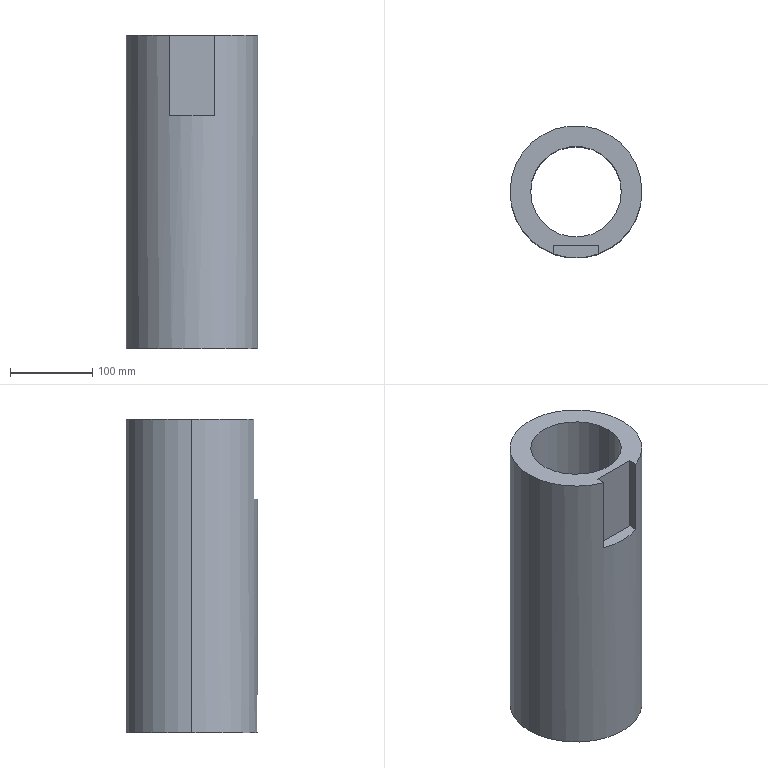Part | SolidWorks | features Cut 2, Extrusion 1 | 1 solid | 10 faces | box 160 x 160 x 380 mm | volume 3957629 mm3 | plane 6 | cylinder 4 | commonest cylinder face diameters 110 x2 160 x2
STEP:
#1=CARTESIAN_POINT('',(-654.884,-90.,0.));
#2=VERTEX_POINT('',#1);
#3=CARTESIAN_POINT('',(-544.884,-90.,0.));
#4=VERTEX_POINT('',#3);
#5=CARTESIAN_POINT('',(-599.884,-90.,0.));
#6=DIRECTION('',(0.,0.,1.));
#7=DIRECTION('',(1.,0.,0.));
#8=AXIS2_PLACEMENT_3D('',#5,#6,#7);
#9=CIRCLE('',#8,55.);
#10=EDGE_CURVE('',#2,#4,#9,.T.);
#11=ORIENTED_EDGE('',*,*,#10,.F.);
#12=CARTESIAN_POINT('',(-654.884,-90.,380.));
#13=VERTEX_POINT('',#12);
#14=CARTESIAN_POINT('',(-654.884,-90.,0.));
#15=DIRECTION('',(0.,0.,1.));
#16=VECTOR('',#15,1000.);
#17=LINE('',#14,#16);
#18=EDGE_CURVE('',#2,#13,#17,.T.);
#19=ORIENTED_EDGE('',*,*,#18,.T.);
#20=CARTESIAN_POINT('',(-544.884,-90.,380.));
#21=VERTEX_POINT('',#20);
#22=CARTESIAN_POINT('',(-599.884,-90.,380.));
#23=DIRECTION('',(0.,0.,1.));
#24=DIRECTION('',(1.,0.,0.));
#25=AXIS2_PLACEMENT_3D('',#22,#23,#24);
#26=CIRCLE('',#25,55.);
#27=EDGE_CURVE('',#13,#21,#26,.T.);
#28=ORIENTED_EDGE('',*,*,#27,.T.);
#29=CARTESIAN_POINT('',(-544.884,-90.,0.));
#30=DIRECTION('',(0.,0.,1.));
#31=VECTOR('',#30,1000.);
#32=LINE('',#29,#31);
#33=EDGE_CURVE('',#4,#21,#32,.T.);
#34=ORIENTED_EDGE('',*,*,#33,.F.);
#35=EDGE_LOOP('',(#11,#19,#28,#34));
#36=FACE_OUTER_BOUND('',#35,.T.);
#37=CARTESIAN_POINT('',(-599.884,-90.,0.));
#38=DIRECTION('',(0.,0.,1.));
#39=DIRECTION('',(1.,0.,0.));
#40=AXIS2_PLACEMENT_3D('',#37,#38,#39);
#41=CYLINDRICAL_SURFACE('',#40,55.);
#42=ADVANCED_FACE('',(#36),#41,.F.);
#43=CARTESIAN_POINT('',(-519.884,-90.,380.));
#44=VERTEX_POINT('',#43);
#45=CARTESIAN_POINT('',(-679.884,-90.,380.));
#46=VERTEX_POINT('',#45);
#47=CARTESIAN_POINT('',(-599.884,-90.,380.));
#48=DIRECTION('',(0.,0.,1.));
#49=DIRECTION('',(1.,0.,0.));
#50=AXIS2_PLACEMENT_3D('',#47,#48,#49);
#51=CIRCLE('',#50,80.);
#52=EDGE_CURVE('',#44,#46,#51,.T.);
#53=ORIENTED_EDGE('',*,*,#52,.F.);
#54=CARTESIAN_POINT('',(-519.884,-90.,0.));
#55=VERTEX_POINT('',#54);
#56=CARTESIAN_POINT('',(-519.884,-90.,380.));
#57=DIRECTION('',(0.,0.,-1.));
#58=VECTOR('',#57,1000.);
#59=LINE('',#56,#58);
#60=EDGE_CURVE('',#44,#55,#59,.T.);
#61=ORIENTED_EDGE('',*,*,#60,.T.);
#62=CARTESIAN_POINT('',(-679.884,-90.,0.));
#63=VERTEX_POINT('',#62);
#64=CARTESIAN_POINT('',(-599.884,-90.,0.));
#65=DIRECTION('',(0.,0.,1.));
#66=DIRECTION('',(1.,0.,0.));
#67=AXIS2_PLACEMENT_3D('',#64,#65,#66);
#68=CIRCLE('',#67,80.);
#69=EDGE_CURVE('',#55,#63,#68,.T.);
#70=ORIENTED_EDGE('',*,*,#69,.T.);
#71=CARTESIAN_POINT('',(-679.884,-90.,380.));
#72=DIRECTION('',(0.,0.,-1.));
#73=VECTOR('',#72,1000.);
#74=LINE('',#71,#73);
#75=EDGE_CURVE('',#46,#63,#74,.T.);
#76=ORIENTED_EDGE('',*,*,#75,.F.);
#77=EDGE_LOOP('',(#53,#61,#70,#76));
#78=FACE_OUTER_BOUND('',#77,.T.);
#79=CARTESIAN_POINT('',(-599.884,-90.,380.));
#80=DIRECTION('',(0.,0.,-1.));
#81=DIRECTION('',(-1.,0.,0.));
#82=AXIS2_PLACEMENT_3D('',#79,#80,#81);
#83=CYLINDRICAL_SURFACE('',#82,80.);
#84=ADVANCED_FACE('',(#78),#83,.T.);
#85=ORIENTED_EDGE('',*,*,#60,.F.);
#86=CARTESIAN_POINT('',(-572.384,-165.125,380.));
#87=VERTEX_POINT('',#86);
#88=CARTESIAN_POINT('',(-599.884,-90.,380.));
#89=DIRECTION('',(0.,0.,1.));
#90=DIRECTION('',(1.,0.,0.));
#91=AXIS2_PLACEMENT_3D('',#88,#89,#90);
#92=CIRCLE('',#91,80.);
#93=EDGE_CURVE('',#87,#44,#92,.T.);
#94=ORIENTED_EDGE('',*,*,#93,.F.);
#95=CARTESIAN_POINT('',(-572.384,-165.125,283.));
#96=VERTEX_POINT('',#95);
#97=CARTESIAN_POINT('',(-572.384,-165.125,283.));
#98=DIRECTION('',(0.,0.,1.));
#99=VECTOR('',#98,1000.);
#100=LINE('',#97,#99);
#101=EDGE_CURVE('',#96,#87,#100,.T.);
#102=ORIENTED_EDGE('',*,*,#101,.F.);
#103=CARTESIAN_POINT('',(-627.384,-165.125,283.));
#104=VERTEX_POINT('',#103);
#105=CARTESIAN_POINT('',(-599.884,-90.,283.));
#106=DIRECTION('',(0.,0.,1.));
#107=DIRECTION('',(1.,0.,0.));
#108=AXIS2_PLACEMENT_3D('',#105,#106,#107);
#109=CIRCLE('',#108,80.);
#110=EDGE_CURVE('',#104,#96,#109,.T.);
#111=ORIENTED_EDGE('',*,*,#110,.F.);
#112=CARTESIAN_POINT('',(-627.384,-165.125,380.));
#113=VERTEX_POINT('',#112);
#114=CARTESIAN_POINT('',(-627.384,-165.125,283.));
#115=DIRECTION('',(0.,0.,1.));
#116=VECTOR('',#115,1000.);
#117=LINE('',#114,#116);
#118=EDGE_CURVE('',#104,#113,#117,.T.);
#119=ORIENTED_EDGE('',*,*,#118,.T.);
#120=CARTESIAN_POINT('',(-599.884,-90.,380.));
#121=DIRECTION('',(0.,0.,1.));
#122=DIRECTION('',(1.,0.,0.));
#123=AXIS2_PLACEMENT_3D('',#120,#121,#122);
#124=CIRCLE('',#123,80.);
#125=EDGE_CURVE('',#46,#113,#124,.T.);
#126=ORIENTED_EDGE('',*,*,#125,.F.);
#127=ORIENTED_EDGE('',*,*,#75,.T.);
#128=CARTESIAN_POINT('',(-599.884,-90.,0.));
#129=DIRECTION('',(0.,0.,1.));
#130=DIRECTION('',(1.,0.,0.));
#131=AXIS2_PLACEMENT_3D('',#128,#129,#130);
#132=CIRCLE('',#131,80.);
#133=EDGE_CURVE('',#63,#55,#132,.T.);
#134=ORIENTED_EDGE('',*,*,#133,.T.);
#135=EDGE_LOOP('',(#85,#94,#102,#111,#119,#126,#127,#134));
#136=FACE_OUTER_BOUND('',#135,.T.);
#137=CARTESIAN_POINT('',(-599.884,-90.,380.));
#138=DIRECTION('',(0.,0.,-1.));
#139=DIRECTION('',(-1.,0.,0.));
#140=AXIS2_PLACEMENT_3D('',#137,#138,#139);
#141=CYLINDRICAL_SURFACE('',#140,80.);
#142=ADVANCED_FACE('',(#136),#141,.T.);
#143=CARTESIAN_POINT('',(-599.884,-90.,380.));
#144=DIRECTION('',(0.,0.,1.));
#145=DIRECTION('',(1.,0.,0.));
#146=AXIS2_PLACEMENT_3D('',#143,#144,#145);
#147=CIRCLE('',#146,55.);
#148=EDGE_CURVE('',#21,#13,#147,.T.);
#149=ORIENTED_EDGE('',*,*,#148,.F.);
#150=ORIENTED_EDGE('',*,*,#27,.F.);
#151=EDGE_LOOP('',(#149,#150));
#152=FACE_BOUND('',#151,.T.);
#153=ORIENTED_EDGE('',*,*,#93,.T.);
#154=ORIENTED_EDGE('',*,*,#52,.T.);
#155=ORIENTED_EDGE('',*,*,#125,.T.);
#156=CARTESIAN_POINT('',(-627.384,-155.,380.));
#157=VERTEX_POINT('',#156);
#158=CARTESIAN_POINT('',(-627.384,0.,380.));
#159=DIRECTION('',(0.,1.,0.));
#160=VECTOR('',#159,1000.);
#161=LINE('',#158,#160);
#162=EDGE_CURVE('',#113,#157,#161,.T.);
#163=ORIENTED_EDGE('',*,*,#162,.T.);
#164=CARTESIAN_POINT('',(-572.384,-155.,380.));
#165=VERTEX_POINT('',#164);
#166=CARTESIAN_POINT('',(0.,-155.,380.));
#167=DIRECTION('',(-1.,0.,0.));
#168=VECTOR('',#167,1000.);
#169=LINE('',#166,#168);
#170=EDGE_CURVE('',#165,#157,#169,.T.);
#171=ORIENTED_EDGE('',*,*,#170,.F.);
#172=CARTESIAN_POINT('',(-572.384,0.,380.));
#173=DIRECTION('',(0.,1.,0.));
#174=VECTOR('',#173,1000.);
#175=LINE('',#172,#174);
#176=EDGE_CURVE('',#87,#165,#175,.T.);
#177=ORIENTED_EDGE('',*,*,#176,.F.);
#178=EDGE_LOOP('',(#153,#154,#155,#163,#171,#177));
#179=FACE_OUTER_BOUND('',#178,.T.);
#180=CARTESIAN_POINT('',(-599.884,-90.,380.));
#181=DIRECTION('',(0.,0.,1.));
#182=DIRECTION('',(1.,0.,0.));
#183=AXIS2_PLACEMENT_3D('',#180,#181,#182);
#184=PLANE('',#183);
#185=ADVANCED_FACE('',(#152,#179),#184,.T.);
#186=CARTESIAN_POINT('',(-599.884,-90.,0.));
#187=DIRECTION('',(0.,0.,1.));
#188=DIRECTION('',(1.,0.,0.));
#189=AXIS2_PLACEMENT_3D('',#186,#187,#188);
#190=CIRCLE('',#189,55.);
#191=EDGE_CURVE('',#4,#2,#190,.T.);
#192=ORIENTED_EDGE('',*,*,#191,.T.);
#193=ORIENTED_EDGE('',*,*,#10,.T.);
#194=EDGE_LOOP('',(#192,#193));
#195=FACE_BOUND('',#194,.T.);
#196=ORIENTED_EDGE('',*,*,#133,.F.);
#197=ORIENTED_EDGE('',*,*,#69,.F.);
#198=EDGE_LOOP('',(#196,#197));
#199=FACE_OUTER_BOUND('',#198,.T.);
#200=CARTESIAN_POINT('',(-599.884,-90.,0.));
#201=DIRECTION('',(0.,0.,1.));
#202=DIRECTION('',(1.,0.,0.));
#203=AXIS2_PLACEMENT_3D('',#200,#201,#202);
#204=PLANE('',#203);
#205=ADVANCED_FACE('',(#195,#199),#204,.F.);
#206=ORIENTED_EDGE('',*,*,#162,.F.);
#207=ORIENTED_EDGE('',*,*,#118,.F.);
#208=CARTESIAN_POINT('',(-627.384,-155.,283.));
#209=VERTEX_POINT('',#208);
#210=CARTESIAN_POINT('',(-627.384,0.,283.));
#211=DIRECTION('',(0.,1.,0.));
#212=VECTOR('',#211,1000.);
#213=LINE('',#210,#212);
#214=EDGE_CURVE('',#104,#209,#213,.T.);
#215=ORIENTED_EDGE('',*,*,#214,.T.);
#216=CARTESIAN_POINT('',(-627.384,-155.,283.));
#217=DIRECTION('',(0.,0.,1.));
#218=VECTOR('',#217,1000.);
#219=LINE('',#216,#218);
#220=EDGE_CURVE('',#209,#157,#219,.T.);
#221=ORIENTED_EDGE('',*,*,#220,.T.);
#222=EDGE_LOOP('',(#206,#207,#215,#221));
#223=FACE_OUTER_BOUND('',#222,.T.);
#224=CARTESIAN_POINT('',(-627.384,0.,283.));
#225=DIRECTION('',(1.,0.,0.));
#226=DIRECTION('',(0.,0.,-1.));
#227=AXIS2_PLACEMENT_3D('',#224,#225,#226);
#228=PLANE('',#227);
#229=ADVANCED_FACE('',(#223),#228,.T.);
#230=ORIENTED_EDGE('',*,*,#170,.T.);
#231=ORIENTED_EDGE('',*,*,#220,.F.);
#232=CARTESIAN_POINT('',(-572.384,-155.,283.));
#233=VERTEX_POINT('',#232);
#234=CARTESIAN_POINT('',(0.,-155.,283.));
#235=DIRECTION('',(-1.,0.,0.));
#236=VECTOR('',#235,1000.);
#237=LINE('',#234,#236);
#238=EDGE_CURVE('',#233,#209,#237,.T.);
#239=ORIENTED_EDGE('',*,*,#238,.F.);
#240=CARTESIAN_POINT('',(-572.384,-155.,283.));
#241=DIRECTION('',(0.,0.,1.));
#242=VECTOR('',#241,1000.);
#243=LINE('',#240,#242);
#244=EDGE_CURVE('',#233,#165,#243,.T.);
#245=ORIENTED_EDGE('',*,*,#244,.T.);
#246=EDGE_LOOP('',(#230,#231,#239,#245));
#247=FACE_OUTER_BOUND('',#246,.T.);
#248=CARTESIAN_POINT('',(0.,-155.,283.));
#249=DIRECTION('',(0.,1.,0.));
#250=DIRECTION('',(0.,0.,1.));
#251=AXIS2_PLACEMENT_3D('',#248,#249,#250);
#252=PLANE('',#251);
#253=ADVANCED_FACE('',(#247),#252,.F.);
#254=ORIENTED_EDGE('',*,*,#176,.T.);
#255=ORIENTED_EDGE('',*,*,#244,.F.);
#256=CARTESIAN_POINT('',(-572.384,0.,283.));
#257=DIRECTION('',(0.,1.,0.));
#258=VECTOR('',#257,1000.);
#259=LINE('',#256,#258);
#260=EDGE_CURVE('',#96,#233,#259,.T.);
#261=ORIENTED_EDGE('',*,*,#260,.F.);
#262=ORIENTED_EDGE('',*,*,#101,.T.);
#263=EDGE_LOOP('',(#254,#255,#261,#262));
#264=FACE_OUTER_BOUND('',#263,.T.);
#265=CARTESIAN_POINT('',(-572.384,0.,283.));
#266=DIRECTION('',(1.,0.,0.));
#267=DIRECTION('',(0.,0.,-1.));
#268=AXIS2_PLACEMENT_3D('',#265,#266,#267);
#269=PLANE('',#268);
#270=ADVANCED_FACE('',(#264),#269,.F.);
#271=ORIENTED_EDGE('',*,*,#214,.F.);
#272=ORIENTED_EDGE('',*,*,#110,.T.);
#273=ORIENTED_EDGE('',*,*,#260,.T.);
#274=ORIENTED_EDGE('',*,*,#238,.T.);
#275=EDGE_LOOP('',(#271,#272,#273,#274));
#276=FACE_OUTER_BOUND('',#275,.T.);
#277=CARTESIAN_POINT('',(0.,0.,283.));
#278=DIRECTION('',(0.,0.,1.));
#279=DIRECTION('',(1.,0.,0.));
#280=AXIS2_PLACEMENT_3D('',#277,#278,#279);
#281=PLANE('',#280);
#282=ADVANCED_FACE('',(#276),#281,.T.);
#283=ORIENTED_EDGE('',*,*,#18,.F.);
#284=ORIENTED_EDGE('',*,*,#191,.F.);
#285=ORIENTED_EDGE('',*,*,#33,.T.);
#286=ORIENTED_EDGE('',*,*,#148,.T.);
#287=EDGE_LOOP('',(#283,#284,#285,#286));
#288=FACE_OUTER_BOUND('',#287,.T.);
#289=CARTESIAN_POINT('',(-599.884,-90.,0.));
#290=DIRECTION('',(0.,0.,1.));
#291=DIRECTION('',(1.,0.,0.));
#292=AXIS2_PLACEMENT_3D('',#289,#290,#291);
#293=CYLINDRICAL_SURFACE('',#292,55.);
#294=ADVANCED_FACE('',(#288),#293,.F.);
#295=CLOSED_SHELL('',(#42,#84,#142,#185,#205,#229,#253,#270,#282,#294));
#296=MANIFOLD_SOLID_BREP('',#295);
#297=CARTESIAN_POINT('',(0.,0.,0.));
#298=DIRECTION('',(0.,0.,1.));
#299=DIRECTION('',(1.,0.,0.));
#300=AXIS2_PLACEMENT_3D('',#297,#298,#299);
#301=(LENGTH_UNIT()NAMED_UNIT(*)SI_UNIT(.MILLI.,.METRE.));
#302=UNCERTAINTY_MEASURE_WITH_UNIT(LENGTH_MEASURE(0.00001),#301,'','');
#303=(NAMED_UNIT(*)PLANE_ANGLE_UNIT()SI_UNIT($,.RADIAN.));
#304=(NAMED_UNIT(*)SI_UNIT($,.STERADIAN.)SOLID_ANGLE_UNIT());
#305=(GEOMETRIC_REPRESENTATION_CONTEXT(3)GLOBAL_UNCERTAINTY_ASSIGNED_CONTEXT((#302))GLOBAL_UNIT_ASSIGNED_CONTEXT((#301,#303,#304))REPRESENTATION_CONTEXT('',''));
#306=ADVANCED_BREP_SHAPE_REPRESENTATION('',(#296,#300),#305);